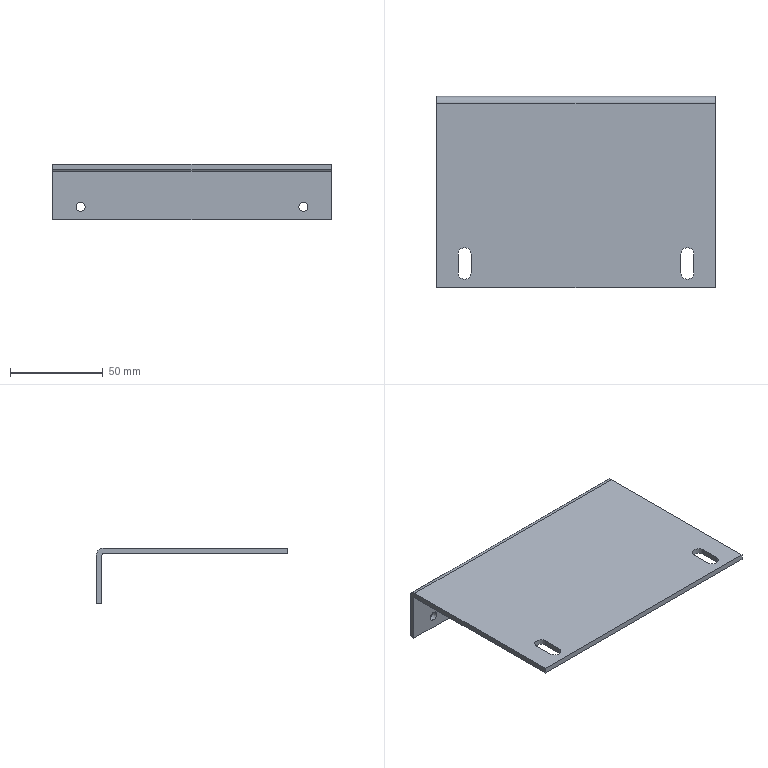Part | STEP file | PN_0035_bracket | 1 solid | 22 faces | box 150 x 103 x 30 mm | volume 57299 mm3 | plane 12 | cylinder 10 | commonest cylinder face diameters 5 x4 7 x4 1.473 x1 7.473 x1